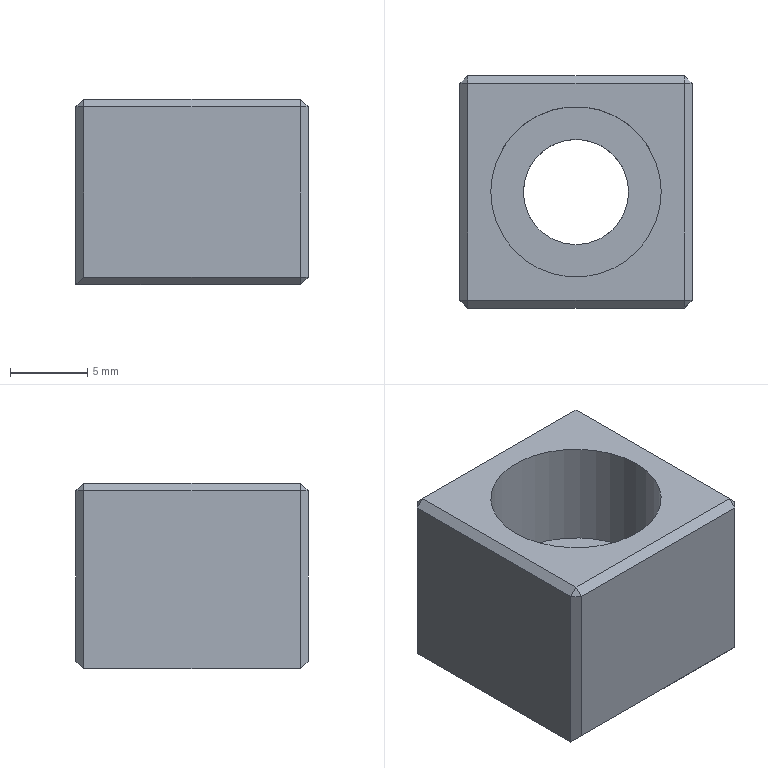Part | NX | features 20 2 | 1 solid | 151 faces | box 15 x 15 x 12 mm | volume 1832 mm3 | plane 125 | spline 24 | cylinder 2 | commonest cylinder face diameters 6.8 x1 11 x1